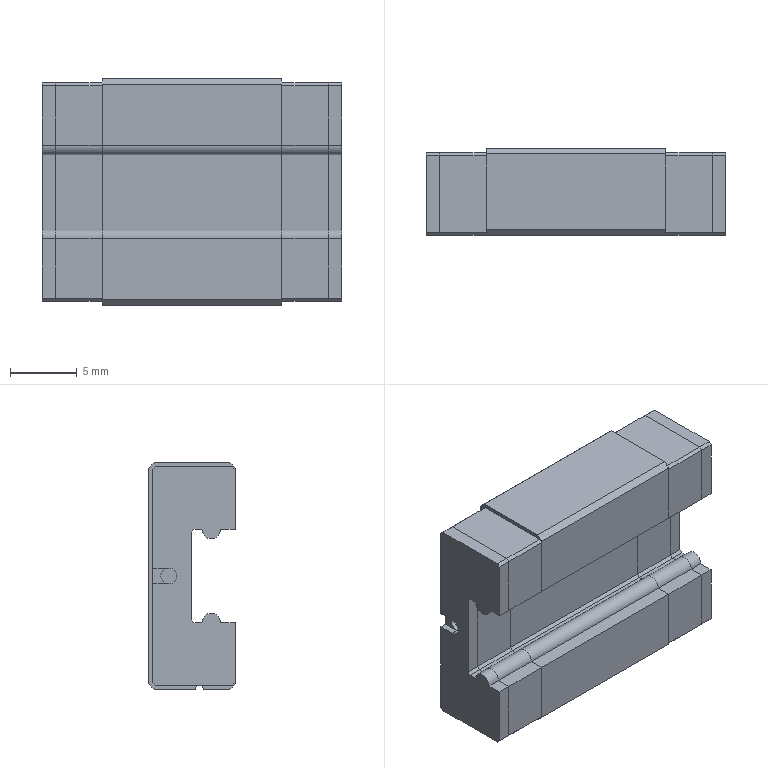Part | SolidWorks | 5 solids | 132 faces | box 22.5 x 6.5 x 17 mm | volume 1884 mm3 | plane 97 | cylinder 27 | cone 8 | commonest cylinder face diameters 1.4 x10 1.2 x8 1.567 x8 0.6 x1